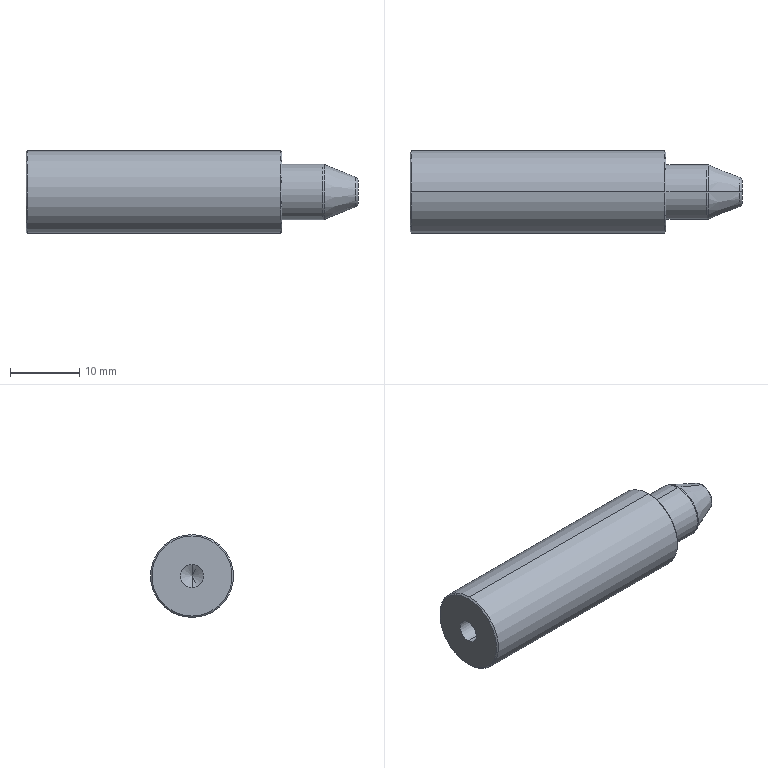Part | STEP file | 1 solid | 21 faces | box 48 x 12 x 12 mm | volume 4513 mm3 | cone 8 | cylinder 6 | torus 4 | plane 3 | commonest cylinder face diameters 3.3 x2 8 x2 12 x2
STEP:
#1=CARTESIAN_POINT('',(0.,0.,0.));
#2=DIRECTION('',(0.,0.,1.));
#3=DIRECTION('',(1.,0.,0.));
#4=AXIS2_PLACEMENT_3D('',#1,#2,#3);
#5=CARTESIAN_POINT('',(42.904,0.,4.));
#6=VERTEX_POINT('',#5);
#7=CARTESIAN_POINT('',(42.904,0.,-4.));
#8=VERTEX_POINT('',#7);
#9=CARTESIAN_POINT('',(42.904,0.,0.));
#10=DIRECTION('',(-1.,0.,0.));
#11=DIRECTION('',(0.,0.,-1.));
#12=AXIS2_PLACEMENT_3D('',#9,#10,#11);
#13=CIRCLE('',#12,4.);
#14=CARTESIAN_POINT('',(42.904,0.,0.));
#15=DIRECTION('',(1.,0.,0.));
#16=DIRECTION('',(0.,0.,-1.));
#17=AXIS2_PLACEMENT_3D('',#14,#15,#16);
#18=TOROIDAL_SURFACE('',#17,3.5,0.5);
#19=CARTESIAN_POINT('',(6.283,0.));
#20=DIRECTION('',(-1.,0.));
#21=VECTOR('',#20,1.);
#22=LINE('',#19,#21);
#23=(GEOMETRIC_REPRESENTATION_CONTEXT(2)PARAMETRIC_REPRESENTATION_CONTEXT()REPRESENTATION_CONTEXT('',''));
#24=DEFINITIONAL_REPRESENTATION('',(#22),#23);
#25=PCURVE('',#18,#24);
#26=CARTESIAN_POINT('',(0.,0.,0.));
#27=DIRECTION('',(-1.,0.,0.));
#28=DIRECTION('',(0.,0.,1.));
#29=AXIS2_PLACEMENT_3D('',#26,#27,#28);
#30=CYLINDRICAL_SURFACE('',#29,4.);
#31=CARTESIAN_POINT('',(-3.142,-42.904));
#32=DIRECTION('',(1.,0.));
#33=VECTOR('',#32,1.);
#34=LINE('',#31,#33);
#35=(GEOMETRIC_REPRESENTATION_CONTEXT(2)PARAMETRIC_REPRESENTATION_CONTEXT()REPRESENTATION_CONTEXT('',''));
#36=DEFINITIONAL_REPRESENTATION('',(#34),#35);
#37=PCURVE('',#30,#36);
#38=SURFACE_CURVE('',#13,(#25,#37),.PCURVE_S1.);
#39=EDGE_CURVE('',#6,#8,#38,.T.);
#40=ORIENTED_EDGE('',*,*,#39,.F.);
#41=CARTESIAN_POINT('',(43.089,0.,3.964));
#42=VERTEX_POINT('',#41);
#43=CARTESIAN_POINT('',(42.904,0.,3.5));
#44=DIRECTION('',(0.,1.,0.));
#45=DIRECTION('',(0.,0.,1.));
#46=AXIS2_PLACEMENT_3D('',#43,#44,#45);
#47=CIRCLE('',#46,0.5);
#48=CARTESIAN_POINT('',(3.142,0.));
#49=DIRECTION('',(0.,1.));
#50=VECTOR('',#49,1.);
#51=LINE('',#48,#50);
#52=(GEOMETRIC_REPRESENTATION_CONTEXT(2)PARAMETRIC_REPRESENTATION_CONTEXT()REPRESENTATION_CONTEXT('',''));
#53=DEFINITIONAL_REPRESENTATION('',(#51),#52);
#54=PCURVE('',#18,#53);
#55=CARTESIAN_POINT('',(42.904,0.,0.));
#56=DIRECTION('',(1.,0.,0.));
#57=DIRECTION('',(0.,0.,-1.));
#58=AXIS2_PLACEMENT_3D('',#55,#56,#57);
#59=TOROIDAL_SURFACE('',#58,3.5,0.5);
#60=CARTESIAN_POINT('',(3.142,0.));
#61=DIRECTION('',(0.,1.));
#62=VECTOR('',#61,1.);
#63=LINE('',#60,#62);
#64=(GEOMETRIC_REPRESENTATION_CONTEXT(2)PARAMETRIC_REPRESENTATION_CONTEXT()REPRESENTATION_CONTEXT('',''));
#65=DEFINITIONAL_REPRESENTATION('',(#63),#64);
#66=PCURVE('',#59,#65);
#67=SURFACE_CURVE('',#47,(#54,#66),.PCURVE_S1.);
#68=EDGE_CURVE('',#6,#42,#67,.T.);
#69=ORIENTED_EDGE('',*,*,#68,.T.);
#70=CARTESIAN_POINT('',(43.089,0.,-3.964));
#71=VERTEX_POINT('',#70);
#72=CARTESIAN_POINT('',(43.089,0.,0.));
#73=DIRECTION('',(1.,0.,0.));
#74=DIRECTION('',(0.,0.,1.));
#75=AXIS2_PLACEMENT_3D('',#72,#73,#74);
#76=CIRCLE('',#75,3.964);
#77=CARTESIAN_POINT('',(-3.142,0.3805));
#78=DIRECTION('',(1.,0.));
#79=VECTOR('',#78,1.);
#80=LINE('',#77,#79);
#81=(GEOMETRIC_REPRESENTATION_CONTEXT(2)PARAMETRIC_REPRESENTATION_CONTEXT()REPRESENTATION_CONTEXT('',''));
#82=DEFINITIONAL_REPRESENTATION('',(#80),#81);
#83=PCURVE('',#18,#82);
#84=CARTESIAN_POINT('',(43.,0.,0.));
#85=DIRECTION('',(-1.,0.,0.));
#86=DIRECTION('',(0.,0.,1.));
#87=AXIS2_PLACEMENT_3D('',#84,#85,#86);
#88=CONICAL_SURFACE('',#87,4.,0.3805);
#89=CARTESIAN_POINT('',(6.283,-0.0894));
#90=DIRECTION('',(-1.,0.));
#91=VECTOR('',#90,1.);
#92=LINE('',#89,#91);
#93=(GEOMETRIC_REPRESENTATION_CONTEXT(2)PARAMETRIC_REPRESENTATION_CONTEXT()REPRESENTATION_CONTEXT('',''));
#94=DEFINITIONAL_REPRESENTATION('',(#92),#93);
#95=PCURVE('',#88,#94);
#96=SURFACE_CURVE('',#76,(#83,#95),.PCURVE_S1.);
#97=EDGE_CURVE('',#71,#42,#96,.T.);
#98=ORIENTED_EDGE('',*,*,#97,.F.);
#99=CARTESIAN_POINT('',(42.904,0.,-3.5));
#100=DIRECTION('',(0.,-1.,0.));
#101=DIRECTION('',(0.,0.,-1.));
#102=AXIS2_PLACEMENT_3D('',#99,#100,#101);
#103=CIRCLE('',#102,0.5);
#104=CARTESIAN_POINT('',(0.,0.));
#105=DIRECTION('',(0.,1.));
#106=VECTOR('',#105,1.);
#107=LINE('',#104,#106);
#108=(GEOMETRIC_REPRESENTATION_CONTEXT(2)PARAMETRIC_REPRESENTATION_CONTEXT()REPRESENTATION_CONTEXT('',''));
#109=DEFINITIONAL_REPRESENTATION('',(#107),#108);
#110=PCURVE('',#18,#109);
#111=CARTESIAN_POINT('',(6.283,0.));
#112=DIRECTION('',(0.,1.));
#113=VECTOR('',#112,1.);
#114=LINE('',#111,#113);
#115=(GEOMETRIC_REPRESENTATION_CONTEXT(2)PARAMETRIC_REPRESENTATION_CONTEXT()REPRESENTATION_CONTEXT('',''));
#116=DEFINITIONAL_REPRESENTATION('',(#114),#115);
#117=PCURVE('',#59,#116);
#118=SURFACE_CURVE('',#103,(#110,#117),.PCURVE_S1.);
#119=EDGE_CURVE('',#8,#71,#118,.T.);
#120=ORIENTED_EDGE('',*,*,#119,.F.);
#121=EDGE_LOOP('',(#40,#69,#98,#120));
#122=FACE_BOUND('',#121,.T.);
#123=ADVANCED_FACE('',(#122),#18,.T.);
#124=CARTESIAN_POINT('',(48.,0.,-1.661));
#125=VERTEX_POINT('',#124);
#126=CARTESIAN_POINT('',(48.,0.,1.661));
#127=VERTEX_POINT('',#126);
#128=CARTESIAN_POINT('',(48.,0.,0.));
#129=DIRECTION('',(1.,0.,0.));
#130=DIRECTION('',(0.,0.,1.));
#131=AXIS2_PLACEMENT_3D('',#128,#129,#130);
#132=CIRCLE('',#131,1.661);
#133=CARTESIAN_POINT('',(47.5,0.,0.));
#134=DIRECTION('',(-1.,0.,0.));
#135=DIRECTION('',(0.,0.,1.));
#136=AXIS2_PLACEMENT_3D('',#133,#134,#135);
#137=TOROIDAL_SURFACE('',#136,1.661,0.5);
#138=CARTESIAN_POINT('',(6.283,4.712));
#139=DIRECTION('',(-1.,0.));
#140=VECTOR('',#139,1.);
#141=LINE('',#138,#140);
#142=(GEOMETRIC_REPRESENTATION_CONTEXT(2)PARAMETRIC_REPRESENTATION_CONTEXT()REPRESENTATION_CONTEXT('',''));
#143=DEFINITIONAL_REPRESENTATION('',(#141),#142);
#144=PCURVE('',#137,#143);
#145=CARTESIAN_POINT('',(48.,0.,0.));
#146=DIRECTION('',(-1.,0.,0.));
#147=DIRECTION('',(0.,0.,1.));
#148=AXIS2_PLACEMENT_3D('',#145,#146,#147);
#149=PLANE('',#148);
#150=CARTESIAN_POINT('',(1.661,0.));
#151=CARTESIAN_POINT('',(1.661,-2.878));
#152=CARTESIAN_POINT('',(-0.8307,-1.439));
#153=CARTESIAN_POINT('',(-3.323,0.));
#154=CARTESIAN_POINT('',(-0.8307,1.439));
#155=CARTESIAN_POINT('',(1.661,2.878));
#156=CARTESIAN_POINT('',(1.661,0.));
#157=(BOUNDED_CURVE()B_SPLINE_CURVE(2,(#150,#151,#152,#153,#154,#155,#156),.UNSPECIFIED.,.T.,.F.)B_SPLINE_CURVE_WITH_KNOTS((1,2,2,2,2,1),(-2.094,0.,2.094,4.189,6.283,8.378),.UNSPECIFIED.)CURVE()GEOMETRIC_REPRESENTATION_ITEM()RATIONAL_B_SPLINE_CURVE((1.,0.5,1.,0.5,1.,0.5,1.))REPRESENTATION_ITEM(''));
#158=(GEOMETRIC_REPRESENTATION_CONTEXT(2)PARAMETRIC_REPRESENTATION_CONTEXT()REPRESENTATION_CONTEXT('',''));
#159=DEFINITIONAL_REPRESENTATION('',(#157),#158);
#160=PCURVE('',#149,#159);
#161=SURFACE_CURVE('',#132,(#144,#160),.PCURVE_S1.);
#162=EDGE_CURVE('',#125,#127,#161,.T.);
#163=ORIENTED_EDGE('',*,*,#162,.F.);
#164=CARTESIAN_POINT('',(47.686,0.,-2.126));
#165=VERTEX_POINT('',#164);
#166=CARTESIAN_POINT('',(47.5,0.,-1.661));
#167=DIRECTION('',(0.,1.,0.));
#168=DIRECTION('',(0.,0.,1.));
#169=AXIS2_PLACEMENT_3D('',#166,#167,#168);
#170=CIRCLE('',#169,0.5);
#171=CARTESIAN_POINT('',(3.142,3.142));
#172=DIRECTION('',(0.,1.));
#173=VECTOR('',#172,1.);
#174=LINE('',#171,#173);
#175=(GEOMETRIC_REPRESENTATION_CONTEXT(2)PARAMETRIC_REPRESENTATION_CONTEXT()REPRESENTATION_CONTEXT('',''));
#176=DEFINITIONAL_REPRESENTATION('',(#174),#175);
#177=PCURVE('',#137,#176);
#178=CARTESIAN_POINT('',(47.5,0.,0.));
#179=DIRECTION('',(-1.,0.,0.));
#180=DIRECTION('',(0.,0.,1.));
#181=AXIS2_PLACEMENT_3D('',#178,#179,#180);
#182=TOROIDAL_SURFACE('',#181,1.661,0.5);
#183=CARTESIAN_POINT('',(3.142,3.142));
#184=DIRECTION('',(0.,1.));
#185=VECTOR('',#184,1.);
#186=LINE('',#183,#185);
#187=(GEOMETRIC_REPRESENTATION_CONTEXT(2)PARAMETRIC_REPRESENTATION_CONTEXT()REPRESENTATION_CONTEXT('',''));
#188=DEFINITIONAL_REPRESENTATION('',(#186),#187);
#189=PCURVE('',#182,#188);
#190=SURFACE_CURVE('',#170,(#177,#189),.PCURVE_S1.);
#191=EDGE_CURVE('',#125,#165,#190,.T.);
#192=ORIENTED_EDGE('',*,*,#191,.T.);
#193=CARTESIAN_POINT('',(47.686,0.,2.126));
#194=VERTEX_POINT('',#193);
#195=CARTESIAN_POINT('',(47.686,0.,0.));
#196=DIRECTION('',(-1.,0.,0.));
#197=DIRECTION('',(0.,0.,1.));
#198=AXIS2_PLACEMENT_3D('',#195,#196,#197);
#199=CIRCLE('',#198,2.126);
#200=CARTESIAN_POINT('',(0.,5.903));
#201=DIRECTION('',(1.,0.));
#202=VECTOR('',#201,1.);
#203=LINE('',#200,#202);
#204=(GEOMETRIC_REPRESENTATION_CONTEXT(2)PARAMETRIC_REPRESENTATION_CONTEXT()REPRESENTATION_CONTEXT('',''));
#205=DEFINITIONAL_REPRESENTATION('',(#203),#204);
#206=PCURVE('',#137,#205);
#207=CARTESIAN_POINT('',(0.,-4.686));
#208=DIRECTION('',(1.,0.));
#209=VECTOR('',#208,1.);
#210=LINE('',#207,#209);
#211=(GEOMETRIC_REPRESENTATION_CONTEXT(2)PARAMETRIC_REPRESENTATION_CONTEXT()REPRESENTATION_CONTEXT('',''));
#212=DEFINITIONAL_REPRESENTATION('',(#210),#211);
#213=PCURVE('',#88,#212);
#214=SURFACE_CURVE('',#199,(#206,#213),.PCURVE_S1.);
#215=EDGE_CURVE('',#194,#165,#214,.T.);
#216=ORIENTED_EDGE('',*,*,#215,.F.);
#217=CARTESIAN_POINT('',(47.5,0.,1.661));
#218=DIRECTION('',(0.,-1.,0.));
#219=DIRECTION('',(0.,0.,-1.));
#220=AXIS2_PLACEMENT_3D('',#217,#218,#219);
#221=CIRCLE('',#220,0.5);
#222=CARTESIAN_POINT('',(0.,3.142));
#223=DIRECTION('',(0.,1.));
#224=VECTOR('',#223,1.);
#225=LINE('',#222,#224);
#226=(GEOMETRIC_REPRESENTATION_CONTEXT(2)PARAMETRIC_REPRESENTATION_CONTEXT()REPRESENTATION_CONTEXT('',''));
#227=DEFINITIONAL_REPRESENTATION('',(#225),#226);
#228=PCURVE('',#137,#227);
#229=CARTESIAN_POINT('',(6.283,3.142));
#230=DIRECTION('',(0.,1.));
#231=VECTOR('',#230,1.);
#232=LINE('',#229,#231);
#233=(GEOMETRIC_REPRESENTATION_CONTEXT(2)PARAMETRIC_REPRESENTATION_CONTEXT()REPRESENTATION_CONTEXT('',''));
#234=DEFINITIONAL_REPRESENTATION('',(#232),#233);
#235=PCURVE('',#182,#234);
#236=SURFACE_CURVE('',#221,(#228,#235),.PCURVE_S1.);
#237=EDGE_CURVE('',#127,#194,#236,.T.);
#238=ORIENTED_EDGE('',*,*,#237,.F.);
#239=EDGE_LOOP('',(#163,#192,#216,#238));
#240=FACE_BOUND('',#239,.T.);
#241=ADVANCED_FACE('',(#240),#137,.T.);
#242=CARTESIAN_POINT('',(37.,0.,-5.8));
#243=VERTEX_POINT('',#242);
#244=CARTESIAN_POINT('',(37.,0.,5.8));
#245=VERTEX_POINT('',#244);
#246=CARTESIAN_POINT('',(37.,0.,0.));
#247=DIRECTION('',(1.,0.,0.));
#248=DIRECTION('',(0.,0.,1.));
#249=AXIS2_PLACEMENT_3D('',#246,#247,#248);
#250=CIRCLE('',#249,5.8);
#251=CARTESIAN_POINT('',(36.8,0.,0.));
#252=DIRECTION('',(-1.,0.,0.));
#253=DIRECTION('',(0.,0.,1.));
#254=AXIS2_PLACEMENT_3D('',#251,#252,#253);
#255=CONICAL_SURFACE('',#254,6.,0.7854);
#256=CARTESIAN_POINT('',(6.283,-0.2));
#257=DIRECTION('',(-1.,0.));
#258=VECTOR('',#257,1.);
#259=LINE('',#256,#258);
#260=(GEOMETRIC_REPRESENTATION_CONTEXT(2)PARAMETRIC_REPRESENTATION_CONTEXT()REPRESENTATION_CONTEXT('',''));
#261=DEFINITIONAL_REPRESENTATION('',(#259),#260);
#262=PCURVE('',#255,#261);
#263=CARTESIAN_POINT('',(37.,4.,0.));
#264=DIRECTION('',(-1.,0.,0.));
#265=DIRECTION('',(0.,0.,1.));
#266=AXIS2_PLACEMENT_3D('',#263,#264,#265);
#267=PLANE('',#266);
#268=CARTESIAN_POINT('',(5.8,-4.));
#269=CARTESIAN_POINT('',(5.8,-14.046));
#270=CARTESIAN_POINT('',(-2.9,-9.023));
#271=CARTESIAN_POINT('',(-11.6,-4.));
#272=CARTESIAN_POINT('',(-2.9,1.023));
#273=CARTESIAN_POINT('',(5.8,6.046));
#274=CARTESIAN_POINT('',(5.8,-4.));
#275=(BOUNDED_CURVE()B_SPLINE_CURVE(2,(#268,#269,#270,#271,#272,#273,#274),.UNSPECIFIED.,.T.,.F.)B_SPLINE_CURVE_WITH_KNOTS((1,2,2,2,2,1),(-2.094,0.,2.094,4.189,6.283,8.378),.UNSPECIFIED.)CURVE()GEOMETRIC_REPRESENTATION_ITEM()RATIONAL_B_SPLINE_CURVE((1.,0.5,1.,0.5,1.,0.5,1.))REPRESENTATION_ITEM(''));
#276=(GEOMETRIC_REPRESENTATION_CONTEXT(2)PARAMETRIC_REPRESENTATION_CONTEXT()REPRESENTATION_CONTEXT('',''));
#277=DEFINITIONAL_REPRESENTATION('',(#275),#276);
#278=PCURVE('',#267,#277);
#279=SURFACE_CURVE('',#250,(#262,#278),.PCURVE_S1.);
#280=EDGE_CURVE('',#243,#245,#279,.T.);
#281=ORIENTED_EDGE('',*,*,#280,.F.);
#282=CARTESIAN_POINT('',(36.8,0.,-6.));
#283=VERTEX_POINT('',#282);
#284=CARTESIAN_POINT('',(36.8,0.,-6.));
#285=DIRECTION('',(-0.7071,0.,-0.7071));
#286=VECTOR('',#285,1.);
#287=LINE('',#284,#286);
#288=CARTESIAN_POINT('',(3.142,0.));
#289=DIRECTION('',(0.,1.));
#290=VECTOR('',#289,1.);
#291=LINE('',#288,#290);
#292=(GEOMETRIC_REPRESENTATION_CONTEXT(2)PARAMETRIC_REPRESENTATION_CONTEXT()REPRESENTATION_CONTEXT('',''));
#293=DEFINITIONAL_REPRESENTATION('',(#291),#292);
#294=PCURVE('',#255,#293);
#295=CARTESIAN_POINT('',(36.8,0.,0.));
#296=DIRECTION('',(-1.,0.,0.));
#297=DIRECTION('',(0.,0.,1.));
#298=AXIS2_PLACEMENT_3D('',#295,#296,#297);
#299=CONICAL_SURFACE('',#298,6.,0.7854);
#300=CARTESIAN_POINT('',(3.142,0.));
#301=DIRECTION('',(0.,1.));
#302=VECTOR('',#301,1.);
#303=LINE('',#300,#302);
#304=(GEOMETRIC_REPRESENTATION_CONTEXT(2)PARAMETRIC_REPRESENTATION_CONTEXT()REPRESENTATION_CONTEXT('',''));
#305=DEFINITIONAL_REPRESENTATION('',(#303),#304);
#306=PCURVE('',#299,#305);
#307=SURFACE_CURVE('',#287,(#294,#306),.PCURVE_S1.);
#308=EDGE_CURVE('',#243,#283,#307,.T.);
#309=ORIENTED_EDGE('',*,*,#308,.T.);
#310=CARTESIAN_POINT('',(36.8,0.,6.));
#311=VERTEX_POINT('',#310);
#312=CARTESIAN_POINT('',(36.8,0.,0.));
#313=DIRECTION('',(-1.,0.,0.));
#314=DIRECTION('',(0.,0.,1.));
#315=AXIS2_PLACEMENT_3D('',#312,#313,#314);
#316=CIRCLE('',#315,6.);
#317=CARTESIAN_POINT('',(0.,0.));
#318=DIRECTION('',(1.,0.));
#319=VECTOR('',#318,1.);
#320=LINE('',#317,#319);
#321=(GEOMETRIC_REPRESENTATION_CONTEXT(2)PARAMETRIC_REPRESENTATION_CONTEXT()REPRESENTATION_CONTEXT('',''));
#322=DEFINITIONAL_REPRESENTATION('',(#320),#321);
#323=PCURVE('',#255,#322);
#324=CARTESIAN_POINT('',(0.,0.,0.));
#325=DIRECTION('',(-1.,0.,0.));
#326=DIRECTION('',(0.,0.,1.));
#327=AXIS2_PLACEMENT_3D('',#324,#325,#326);
#328=CYLINDRICAL_SURFACE('',#327,6.);
#329=CARTESIAN_POINT('',(0.,-36.8));
#330=DIRECTION('',(1.,0.));
#331=VECTOR('',#330,1.);
#332=LINE('',#329,#331);
#333=(GEOMETRIC_REPRESENTATION_CONTEXT(2)PARAMETRIC_REPRESENTATION_CONTEXT()REPRESENTATION_CONTEXT('',''));
#334=DEFINITIONAL_REPRESENTATION('',(#332),#333);
#335=PCURVE('',#328,#334);
#336=SURFACE_CURVE('',#316,(#323,#335),.PCURVE_S1.);
#337=EDGE_CURVE('',#311,#283,#336,.T.);
#338=ORIENTED_EDGE('',*,*,#337,.F.);
#339=CARTESIAN_POINT('',(36.8,0.,6.));
#340=DIRECTION('',(-0.7071,0.,0.7071));
#341=VECTOR('',#340,1.);
#342=LINE('',#339,#341);
#343=CARTESIAN_POINT('',(0.,0.));
#344=DIRECTION('',(0.,1.));
#345=VECTOR('',#344,1.);
#346=LINE('',#343,#345);
#347=(GEOMETRIC_REPRESENTATION_CONTEXT(2)PARAMETRIC_REPRESENTATION_CONTEXT()REPRESENTATION_CONTEXT('',''));
#348=DEFINITIONAL_REPRESENTATION('',(#346),#347);
#349=PCURVE('',#255,#348);
#350=CARTESIAN_POINT('',(6.283,0.));
#351=DIRECTION('',(0.,1.));
#352=VECTOR('',#351,1.);
#353=LINE('',#350,#352);
#354=(GEOMETRIC_REPRESENTATION_CONTEXT(2)PARAMETRIC_REPRESENTATION_CONTEXT()REPRESENTATION_CONTEXT('',''));
#355=DEFINITIONAL_REPRESENTATION('',(#353),#354);
#356=PCURVE('',#299,#355);
#357=SURFACE_CURVE('',#342,(#349,#356),.PCURVE_S1.);
#358=EDGE_CURVE('',#245,#311,#357,.T.);
#359=ORIENTED_EDGE('',*,*,#358,.F.);
#360=EDGE_LOOP('',(#281,#309,#338,#359));
#361=FACE_BOUND('',#360,.T.);
#362=ADVANCED_FACE('',(#361),#255,.T.);
#363=CARTESIAN_POINT('',(0.,0.,5.8));
#364=VERTEX_POINT('',#363);
#365=CARTESIAN_POINT('',(0.,0.,-5.8));
#366=VERTEX_POINT('',#365);
#367=CARTESIAN_POINT('',(0.,0.,0.));
#368=DIRECTION('',(-1.,0.,0.));
#369=DIRECTION('',(0.,0.,-1.));
#370=AXIS2_PLACEMENT_3D('',#367,#368,#369);
#371=CIRCLE('',#370,5.8);
#372=CARTESIAN_POINT('',(0.,0.,0.));
#373=DIRECTION('',(1.,0.,0.));
#374=DIRECTION('',(0.,0.,-1.));
#375=AXIS2_PLACEMENT_3D('',#372,#373,#374);
#376=CONICAL_SURFACE('',#375,5.8,0.7854);
#377=CARTESIAN_POINT('',(6.283,0.));
#378=DIRECTION('',(-1.,0.));
#379=VECTOR('',#378,1.);
#380=LINE('',#377,#379);
#381=(GEOMETRIC_REPRESENTATION_CONTEXT(2)PARAMETRIC_REPRESENTATION_CONTEXT()REPRESENTATION_CONTEXT('',''));
#382=DEFINITIONAL_REPRESENTATION('',(#380),#381);
#383=PCURVE('',#376,#382);
#384=CARTESIAN_POINT('',(0.,6.,0.));
#385=DIRECTION('',(1.,0.,0.));
#386=DIRECTION('',(0.,0.,-1.));
#387=AXIS2_PLACEMENT_3D('',#384,#385,#386);
#388=PLANE('',#387);
#389=CARTESIAN_POINT('',(5.8,-6.));
#390=CARTESIAN_POINT('',(5.8,-16.046));
#391=CARTESIAN_POINT('',(-2.9,-11.023));
#392=CARTESIAN_POINT('',(-11.6,-6.));
#393=CARTESIAN_POINT('',(-2.9,-0.9771));
#394=CARTESIAN_POINT('',(5.8,4.046));
#395=CARTESIAN_POINT('',(5.8,-6.));
#396=(BOUNDED_CURVE()B_SPLINE_CURVE(2,(#389,#390,#391,#392,#393,#394,#395),.UNSPECIFIED.,.T.,.F.)B_SPLINE_CURVE_WITH_KNOTS((1,2,2,2,2,1),(-2.094,0.,2.094,4.189,6.283,8.378),.UNSPECIFIED.)CURVE()GEOMETRIC_REPRESENTATION_ITEM()RATIONAL_B_SPLINE_CURVE((1.,0.5,1.,0.5,1.,0.5,1.))REPRESENTATION_ITEM(''));
#397=(GEOMETRIC_REPRESENTATION_CONTEXT(2)PARAMETRIC_REPRESENTATION_CONTEXT()REPRESENTATION_CONTEXT('',''));
#398=DEFINITIONAL_REPRESENTATION('',(#396),#397);
#399=PCURVE('',#388,#398);
#400=SURFACE_CURVE('',#371,(#383,#399),.PCURVE_S1.);
#401=EDGE_CURVE('',#364,#366,#400,.T.);
#402=ORIENTED_EDGE('',*,*,#401,.F.);
#403=CARTESIAN_POINT('',(0.2,0.,6.));
#404=VERTEX_POINT('',#403);
#405=CARTESIAN_POINT('',(0.,0.,5.8));
#406=DIRECTION('',(0.7071,0.,0.7071));
#407=VECTOR('',#406,1.);
#408=LINE('',#405,#407);
#409=CARTESIAN_POINT('',(3.142,0.));
#410=DIRECTION('',(0.,1.));
#411=VECTOR('',#410,1.);
#412=LINE('',#409,#411);
#413=(GEOMETRIC_REPRESENTATION_CONTEXT(2)PARAMETRIC_REPRESENTATION_CONTEXT()REPRESENTATION_CONTEXT('',''));
#414=DEFINITIONAL_REPRESENTATION('',(#412),#413);
#415=PCURVE('',#376,#414);
#416=CARTESIAN_POINT('',(0.,0.,0.));
#417=DIRECTION('',(1.,0.,0.));
#418=DIRECTION('',(0.,0.,-1.));
#419=AXIS2_PLACEMENT_3D('',#416,#417,#418);
#420=CONICAL_SURFACE('',#419,5.8,0.7854);
#421=CARTESIAN_POINT('',(3.142,0.));
#422=DIRECTION('',(0.,1.));
#423=VECTOR('',#422,1.);
#424=LINE('',#421,#423);
#425=(GEOMETRIC_REPRESENTATION_CONTEXT(2)PARAMETRIC_REPRESENTATION_CONTEXT()REPRESENTATION_CONTEXT('',''));
#426=DEFINITIONAL_REPRESENTATION('',(#424),#425);
#427=PCURVE('',#420,#426);
#428=SURFACE_CURVE('',#408,(#415,#427),.PCURVE_S1.);
#429=EDGE_CURVE('',#364,#404,#428,.T.);
#430=ORIENTED_EDGE('',*,*,#429,.T.);
#431=CARTESIAN_POINT('',(0.2,0.,-6.));
#432=VERTEX_POINT('',#431);
#433=CARTESIAN_POINT('',(0.2,0.,0.));
#434=DIRECTION('',(1.,0.,0.));
#435=DIRECTION('',(0.,0.,-1.));
#436=AXIS2_PLACEMENT_3D('',#433,#434,#435);
#437=CIRCLE('',#436,6.);
#438=CARTESIAN_POINT('',(0.,0.2));
#439=DIRECTION('',(1.,0.));
#440=VECTOR('',#439,1.);
#441=LINE('',#438,#440);
#442=(GEOMETRIC_REPRESENTATION_CONTEXT(2)PARAMETRIC_REPRESENTATION_CONTEXT()REPRESENTATION_CONTEXT('',''));
#443=DEFINITIONAL_REPRESENTATION('',(#441),#442);
#444=PCURVE('',#376,#443);
#445=CARTESIAN_POINT('',(3.142,-0.2));
#446=DIRECTION('',(-1.,0.));
#447=VECTOR('',#446,1.);
#448=LINE('',#445,#447);
#449=(GEOMETRIC_REPRESENTATION_CONTEXT(2)PARAMETRIC_REPRESENTATION_CONTEXT()REPRESENTATION_CONTEXT('',''));
#450=DEFINITIONAL_REPRESENTATION('',(#448),#449);
#451=PCURVE('',#328,#450);
#452=SURFACE_CURVE('',#437,(#444,#451),.PCURVE_S1.);
#453=EDGE_CURVE('',#432,#404,#452,.T.);
#454=ORIENTED_EDGE('',*,*,#453,.F.);
#455=CARTESIAN_POINT('',(0.,0.,-5.8));
#456=DIRECTION('',(0.7071,0.,-0.7071));
#457=VECTOR('',#456,1.);
#458=LINE('',#455,#457);
#459=CARTESIAN_POINT('',(0.,0.));
#460=DIRECTION('',(0.,1.));
#461=VECTOR('',#460,1.);
#462=LINE('',#459,#461);
#463=(GEOMETRIC_REPRESENTATION_CONTEXT(2)PARAMETRIC_REPRESENTATION_CONTEXT()REPRESENTATION_CONTEXT('',''));
#464=DEFINITIONAL_REPRESENTATION('',(#462),#463);
#465=PCURVE('',#376,#464);
#466=CARTESIAN_POINT('',(6.283,0.));
#467=DIRECTION('',(0.,1.));
#468=VECTOR('',#467,1.);
#469=LINE('',#466,#468);
#470=(GEOMETRIC_REPRESENTATION_CONTEXT(2)PARAMETRIC_REPRESENTATION_CONTEXT()REPRESENTATION_CONTEXT('',''));
#471=DEFINITIONAL_REPRESENTATION('',(#469),#470);
#472=PCURVE('',#420,#471);
#473=SURFACE_CURVE('',#458,(#465,#472),.PCURVE_S1.);
#474=EDGE_CURVE('',#366,#432,#473,.T.);
#475=ORIENTED_EDGE('',*,*,#474,.F.);
#476=EDGE_LOOP('',(#402,#430,#454,#475));
#477=FACE_BOUND('',#476,.T.);
#478=ADVANCED_FACE('',(#477),#376,.T.);
#479=ORIENTED_EDGE('',*,*,#215,.T.);
#480=CARTESIAN_POINT('',(43.,0.,-4.));
#481=DIRECTION('',(-0.9285,0.,-0.3714));
#482=VECTOR('',#481,1.);
#483=LINE('',#480,#482);
#484=CARTESIAN_POINT('',(3.142,0.));
#485=DIRECTION('',(0.,1.));
#486=VECTOR('',#485,1.);
#487=LINE('',#484,#486);
#488=(GEOMETRIC_REPRESENTATION_CONTEXT(2)PARAMETRIC_REPRESENTATION_CONTEXT()REPRESENTATION_CONTEXT('',''));
#489=DEFINITIONAL_REPRESENTATION('',(#487),#488);
#490=PCURVE('',#88,#489);
#491=CARTESIAN_POINT('',(43.,0.,0.));
#492=DIRECTION('',(-1.,0.,0.));
#493=DIRECTION('',(0.,0.,1.));
#494=AXIS2_PLACEMENT_3D('',#491,#492,#493);
#495=CONICAL_SURFACE('',#494,4.,0.3805);
#496=CARTESIAN_POINT('',(3.142,0.));
#497=DIRECTION('',(0.,1.));
#498=VECTOR('',#497,1.);
#499=LINE('',#496,#498);
#500=(GEOMETRIC_REPRESENTATION_CONTEXT(2)PARAMETRIC_REPRESENTATION_CONTEXT()REPRESENTATION_CONTEXT('',''));
#501=DEFINITIONAL_REPRESENTATION('',(#499),#500);
#502=PCURVE('',#495,#501);
#503=SURFACE_CURVE('',#483,(#490,#502),.PCURVE_S1.);
#504=EDGE_CURVE('',#165,#71,#503,.T.);
#505=ORIENTED_EDGE('',*,*,#504,.T.);
#506=ORIENTED_EDGE('',*,*,#97,.T.);
#507=CARTESIAN_POINT('',(43.,0.,4.));
#508=DIRECTION('',(-0.9285,0.,0.3714));
#509=VECTOR('',#508,1.);
#510=LINE('',#507,#509);
#511=CARTESIAN_POINT('',(0.,0.));
#512=DIRECTION('',(0.,1.));
#513=VECTOR('',#512,1.);
#514=LINE('',#511,#513);
#515=(GEOMETRIC_REPRESENTATION_CONTEXT(2)PARAMETRIC_REPRESENTATION_CONTEXT()REPRESENTATION_CONTEXT('',''));
#516=DEFINITIONAL_REPRESENTATION('',(#514),#515);
#517=PCURVE('',#88,#516);
#518=CARTESIAN_POINT('',(6.283,0.));
#519=DIRECTION('',(0.,1.));
#520=VECTOR('',#519,1.);
#521=LINE('',#518,#520);
#522=(GEOMETRIC_REPRESENTATION_CONTEXT(2)PARAMETRIC_REPRESENTATION_CONTEXT()REPRESENTATION_CONTEXT('',''));
#523=DEFINITIONAL_REPRESENTATION('',(#521),#522);
#524=PCURVE('',#495,#523);
#525=SURFACE_CURVE('',#510,(#517,#524),.PCURVE_S1.);
#526=EDGE_CURVE('',#194,#42,#525,.T.);
#527=ORIENTED_EDGE('',*,*,#526,.F.);
#528=EDGE_LOOP('',(#479,#505,#506,#527));
#529=FACE_BOUND('',#528,.T.);
#530=ADVANCED_FACE('',(#529),#88,.T.);
#531=CARTESIAN_POINT('',(13.5,0.,1.65));
#532=VERTEX_POINT('',#531);
#533=CARTESIAN_POINT('',(0.,0.,1.65));
#534=VERTEX_POINT('',#533);
#535=CARTESIAN_POINT('',(0.,0.,1.65));
#536=DIRECTION('',(-1.,0.,0.));
#537=VECTOR('',#536,1.);
#538=LINE('',#535,#537);
#539=CARTESIAN_POINT('',(0.,0.,0.));
#540=DIRECTION('',(-1.,0.,0.));
#541=DIRECTION('',(0.,0.,1.));
#542=AXIS2_PLACEMENT_3D('',#539,#540,#541);
#543=CYLINDRICAL_SURFACE('',#542,1.65);
#544=CARTESIAN_POINT('',(6.283,0.));
#545=DIRECTION('',(0.,1.));
#546=VECTOR('',#545,1.);
#547=LINE('',#544,#546);
#548=(GEOMETRIC_REPRESENTATION_CONTEXT(2)PARAMETRIC_REPRESENTATION_CONTEXT()REPRESENTATION_CONTEXT('',''));
#549=DEFINITIONAL_REPRESENTATION('',(#547),#548);
#550=PCURVE('',#543,#549);
#551=CARTESIAN_POINT('',(0.,0.,0.));
#552=DIRECTION('',(-1.,0.,0.));
#553=DIRECTION('',(0.,0.,1.));
#554=AXIS2_PLACEMENT_3D('',#551,#552,#553);
#555=CYLINDRICAL_SURFACE('',#554,1.65);
#556=CARTESIAN_POINT('',(0.,0.));
#557=DIRECTION('',(0.,1.));
#558=VECTOR('',#557,1.);
#559=LINE('',#556,#558);
#560=(GEOMETRIC_REPRESENTATION_CONTEXT(2)PARAMETRIC_REPRESENTATION_CONTEXT()REPRESENTATION_CONTEXT('',''));
#561=DEFINITIONAL_REPRESENTATION('',(#559),#560);
#562=PCURVE('',#555,#561);
#563=SURFACE_CURVE('',#538,(#550,#562),.PCURVE_S1.);
#564=EDGE_CURVE('',#532,#534,#563,.T.);
#565=ORIENTED_EDGE('',*,*,#564,.T.);
#566=CARTESIAN_POINT('',(0.,0.,-1.65));
#567=VERTEX_POINT('',#566);
#568=CARTESIAN_POINT('',(0.,0.,0.));
#569=DIRECTION('',(-1.,0.,0.));
#570=DIRECTION('',(0.,0.,1.));
#571=AXIS2_PLACEMENT_3D('',#568,#569,#570);
#572=CIRCLE('',#571,1.65);
#573=CARTESIAN_POINT('',(0.,0.));
#574=DIRECTION('',(1.,0.));
#575=VECTOR('',#574,1.);
#576=LINE('',#573,#575);
#577=(GEOMETRIC_REPRESENTATION_CONTEXT(2)PARAMETRIC_REPRESENTATION_CONTEXT()REPRESENTATION_CONTEXT('',''));
#578=DEFINITIONAL_REPRESENTATION('',(#576),#577);
#579=PCURVE('',#543,#578);
#580=CARTESIAN_POINT('',(-1.65,-6.));
#581=CARTESIAN_POINT('',(-1.65,-3.142));
#582=CARTESIAN_POINT('',(0.825,-4.571));
#583=CARTESIAN_POINT('',(3.3,-6.));
#584=CARTESIAN_POINT('',(0.825,-7.429));
#585=CARTESIAN_POINT('',(-1.65,-8.858));
#586=CARTESIAN_POINT('',(-1.65,-6.));
#587=(BOUNDED_CURVE()B_SPLINE_CURVE(2,(#580,#581,#582,#583,#584,#585,#586),.UNSPECIFIED.,.T.,.F.)B_SPLINE_CURVE_WITH_KNOTS((1,2,2,2,2,1),(-2.094,0.,2.094,4.189,6.283,8.378),.UNSPECIFIED.)CURVE()GEOMETRIC_REPRESENTATION_ITEM()RATIONAL_B_SPLINE_CURVE((1.,0.5,1.,0.5,1.,0.5,1.))REPRESENTATION_ITEM(''));
#588=(GEOMETRIC_REPRESENTATION_CONTEXT(2)PARAMETRIC_REPRESENTATION_CONTEXT()REPRESENTATION_CONTEXT('',''));
#589=DEFINITIONAL_REPRESENTATION('',(#587),#588);
#590=PCURVE('',#388,#589);
#591=SURFACE_CURVE('',#572,(#579,#590),.PCURVE_S1.);
#592=EDGE_CURVE('',#567,#534,#591,.T.);
#593=ORIENTED_EDGE('',*,*,#592,.F.);
#594=CARTESIAN_POINT('',(13.5,0.,-1.65));
#595=VERTEX_POINT('',#594);
#596=CARTESIAN_POINT('',(0.,0.,-1.65));
#597=DIRECTION('',(-1.,0.,0.));
#598=VECTOR('',#597,1.);
#599=LINE('',#596,#598);
#600=CARTESIAN_POINT('',(3.142,0.));
#601=DIRECTION('',(0.,1.));
#602=VECTOR('',#601,1.);
#603=LINE('',#600,#602);
#604=(GEOMETRIC_REPRESENTATION_CONTEXT(2)PARAMETRIC_REPRESENTATION_CONTEXT()REPRESENTATION_CONTEXT('',''));
#605=DEFINITIONAL_REPRESENTATION('',(#603),#604);
#606=PCURVE('',#543,#605);
#607=CARTESIAN_POINT('',(3.142,0.));
#608=DIRECTION('',(0.,1.));
#609=VECTOR('',#608,1.);
#610=LINE('',#607,#609);
#611=(GEOMETRIC_REPRESENTATION_CONTEXT(2)PARAMETRIC_REPRESENTATION_CONTEXT()REPRESENTATION_CONTEXT('',''));
#612=DEFINITIONAL_REPRESENTATION('',(#610),#611);
#613=PCURVE('',#555,#612);
#614=SURFACE_CURVE('',#599,(#606,#613),.PCURVE_S1.);
#615=EDGE_CURVE('',#595,#567,#614,.T.);
#616=ORIENTED_EDGE('',*,*,#615,.F.);
#617=CARTESIAN_POINT('',(13.5,0.,0.));
#618=DIRECTION('',(-1.,0.,0.));
#619=DIRECTION('',(0.,0.,1.));
#620=AXIS2_PLACEMENT_3D('',#617,#618,#619);
#621=CIRCLE('',#620,1.65);
#622=CARTESIAN_POINT('',(0.,-13.5));
#623=DIRECTION('',(1.,0.));
#624=VECTOR('',#623,1.);
#625=LINE('',#622,#624);
#626=(GEOMETRIC_REPRESENTATION_CONTEXT(2)PARAMETRIC_REPRESENTATION_CONTEXT()REPRESENTATION_CONTEXT('',''));
#627=DEFINITIONAL_REPRESENTATION('',(#625),#626);
#628=PCURVE('',#543,#627);
#629=CARTESIAN_POINT('',(13.5,0.,0.));
#630=DIRECTION('',(-1.,0.,0.));
#631=DIRECTION('',(0.,0.,1.));
#632=AXIS2_PLACEMENT_3D('',#629,#630,#631);
#633=CONICAL_SURFACE('',#632,1.65,1.03);
#634=CARTESIAN_POINT('',(0.,0.));
#635=DIRECTION('',(1.,0.));
#636=VECTOR('',#635,1.);
#637=LINE('',#634,#636);
#638=(GEOMETRIC_REPRESENTATION_CONTEXT(2)PARAMETRIC_REPRESENTATION_CONTEXT()REPRESENTATION_CONTEXT('',''));
#639=DEFINITIONAL_REPRESENTATION('',(#637),#638);
#640=PCURVE('',#633,#639);
#641=SURFACE_CURVE('',#621,(#628,#640),.PCURVE_S1.);
#642=EDGE_CURVE('',#595,#532,#641,.T.);
#643=ORIENTED_EDGE('',*,*,#642,.T.);
#644=EDGE_LOOP('',(#565,#593,#616,#643));
#645=FACE_BOUND('',#644,.F.);
#646=ADVANCED_FACE('',(#645),#543,.F.);
#647=ORIENTED_EDGE('',*,*,#642,.F.);
#648=CARTESIAN_POINT('',(14.491,0.,0.));
#649=VERTEX_POINT('',#648);
#650=CARTESIAN_POINT('',(13.5,0.,-1.65));
#651=DIRECTION('',(-0.515,0.,-0.8572));
#652=VECTOR('',#651,1.);
#653=LINE('',#650,#652);
#654=CARTESIAN_POINT('',(3.142,0.));
#655=DIRECTION('',(0.,1.));
#656=VECTOR('',#655,1.);
#657=LINE('',#654,#656);
#658=(GEOMETRIC_REPRESENTATION_CONTEXT(2)PARAMETRIC_REPRESENTATION_CONTEXT()REPRESENTATION_CONTEXT('',''));
#659=DEFINITIONAL_REPRESENTATION('',(#657),#658);
#660=PCURVE('',#633,#659);
#661=CARTESIAN_POINT('',(13.5,0.,0.));
#662=DIRECTION('',(-1.,0.,0.));
#663=DIRECTION('',(0.,0.,1.));
#664=AXIS2_PLACEMENT_3D('',#661,#662,#663);
#665=CONICAL_SURFACE('',#664,1.65,1.03);
#666=CARTESIAN_POINT('',(3.142,0.));
#667=DIRECTION('',(0.,1.));
#668=VECTOR('',#667,1.);
#669=LINE('',#666,#668);
#670=(GEOMETRIC_REPRESENTATION_CONTEXT(2)PARAMETRIC_REPRESENTATION_CONTEXT()REPRESENTATION_CONTEXT('',''));
#671=DEFINITIONAL_REPRESENTATION('',(#669),#670);
#672=PCURVE('',#665,#671);
#673=SURFACE_CURVE('',#653,(#660,#672),.PCURVE_S1.);
#674=EDGE_CURVE('',#649,#595,#673,.T.);
#675=ORIENTED_EDGE('',*,*,#674,.F.);
#676=CARTESIAN_POINT('',(13.5,0.,1.65));
#677=DIRECTION('',(-0.515,0.,0.8572));
#678=VECTOR('',#677,1.);
#679=LINE('',#676,#678);
#680=CARTESIAN_POINT('',(6.283,0.));
#681=DIRECTION('',(0.,1.));
#682=VECTOR('',#681,1.);
#683=LINE('',#680,#682);
#684=(GEOMETRIC_REPRESENTATION_CONTEXT(2)PARAMETRIC_REPRESENTATION_CONTEXT()REPRESENTATION_CONTEXT('',''));
#685=DEFINITIONAL_REPRESENTATION('',(#683),#684);
#686=PCURVE('',#633,#685);
#687=CARTESIAN_POINT('',(0.,0.));
#688=DIRECTION('',(0.,1.));
#689=VECTOR('',#688,1.);
#690=LINE('',#687,#689);
#691=(GEOMETRIC_REPRESENTATION_CONTEXT(2)PARAMETRIC_REPRESENTATION_CONTEXT()REPRESENTATION_CONTEXT('',''));
#692=DEFINITIONAL_REPRESENTATION('',(#690),#691);
#693=PCURVE('',#665,#692);
#694=SURFACE_CURVE('',#679,(#686,#693),.PCURVE_S1.);
#695=EDGE_CURVE('',#649,#532,#694,.T.);
#696=ORIENTED_EDGE('',*,*,#695,.T.);
#697=EDGE_LOOP('',(#647,#675,#696));
#698=FACE_BOUND('',#697,.F.);
#699=ADVANCED_FACE('',(#698),#633,.F.);
#700=ORIENTED_EDGE('',*,*,#337,.T.);
#701=CARTESIAN_POINT('',(0.,0.,-6.));
#702=DIRECTION('',(-1.,0.,0.));
#703=VECTOR('',#702,1.);
#704=LINE('',#701,#703);
#705=CARTESIAN_POINT('',(3.142,0.));
#706=DIRECTION('',(0.,1.));
#707=VECTOR('',#706,1.);
#708=LINE('',#705,#707);
#709=(GEOMETRIC_REPRESENTATION_CONTEXT(2)PARAMETRIC_REPRESENTATION_CONTEXT()REPRESENTATION_CONTEXT('',''));
#710=DEFINITIONAL_REPRESENTATION('',(#708),#709);
#711=PCURVE('',#328,#710);
#712=CARTESIAN_POINT('',(0.,0.,0.));
#713=DIRECTION('',(-1.,0.,0.));
#714=DIRECTION('',(0.,0.,1.));
#715=AXIS2_PLACEMENT_3D('',#712,#713,#714);
#716=CYLINDRICAL_SURFACE('',#715,6.);
#717=CARTESIAN_POINT('',(3.142,0.));
#718=DIRECTION('',(0.,1.));
#719=VECTOR('',#718,1.);
#720=LINE('',#717,#719);
#721=(GEOMETRIC_REPRESENTATION_CONTEXT(2)PARAMETRIC_REPRESENTATION_CONTEXT()REPRESENTATION_CONTEXT('',''));
#722=DEFINITIONAL_REPRESENTATION('',(#720),#721);
#723=PCURVE('',#716,#722);
#724=SURFACE_CURVE('',#704,(#711,#723),.PCURVE_S1.);
#725=EDGE_CURVE('',#283,#432,#724,.T.);
#726=ORIENTED_EDGE('',*,*,#725,.T.);
#727=ORIENTED_EDGE('',*,*,#453,.T.);
#728=CARTESIAN_POINT('',(0.,0.,6.));
#729=DIRECTION('',(-1.,0.,0.));
#730=VECTOR('',#729,1.);
#731=LINE('',#728,#730);
#732=CARTESIAN_POINT('',(0.,0.));
#733=DIRECTION('',(0.,1.));
#734=VECTOR('',#733,1.);
#735=LINE('',#732,#734);
#736=(GEOMETRIC_REPRESENTATION_CONTEXT(2)PARAMETRIC_REPRESENTATION_CONTEXT()REPRESENTATION_CONTEXT('',''));
#737=DEFINITIONAL_REPRESENTATION('',(#735),#736);
#738=PCURVE('',#328,#737);
#739=CARTESIAN_POINT('',(6.283,0.));
#740=DIRECTION('',(0.,1.));
#741=VECTOR('',#740,1.);
#742=LINE('',#739,#741);
#743=(GEOMETRIC_REPRESENTATION_CONTEXT(2)PARAMETRIC_REPRESENTATION_CONTEXT()REPRESENTATION_CONTEXT('',''));
#744=DEFINITIONAL_REPRESENTATION('',(#742),#743);
#745=PCURVE('',#716,#744);
#746=SURFACE_CURVE('',#731,(#738,#745),.PCURVE_S1.);
#747=EDGE_CURVE('',#311,#404,#746,.T.);
#748=ORIENTED_EDGE('',*,*,#747,.F.);
#749=EDGE_LOOP('',(#700,#726,#727,#748));
#750=FACE_BOUND('',#749,.T.);
#751=ADVANCED_FACE('',(#750),#328,.T.);
#752=ORIENTED_EDGE('',*,*,#39,.T.);
#753=CARTESIAN_POINT('',(37.,0.,-4.));
#754=VERTEX_POINT('',#753);
#755=CARTESIAN_POINT('',(0.,0.,-4.));
#756=DIRECTION('',(-1.,0.,0.));
#757=VECTOR('',#756,1.);
#758=LINE('',#755,#757);
#759=CARTESIAN_POINT('',(3.142,0.));
#760=DIRECTION('',(0.,1.));
#761=VECTOR('',#760,1.);
#762=LINE('',#759,#761);
#763=(GEOMETRIC_REPRESENTATION_CONTEXT(2)PARAMETRIC_REPRESENTATION_CONTEXT()REPRESENTATION_CONTEXT('',''));
#764=DEFINITIONAL_REPRESENTATION('',(#762),#763);
#765=PCURVE('',#30,#764);
#766=CARTESIAN_POINT('',(0.,0.,0.));
#767=DIRECTION('',(-1.,0.,0.));
#768=DIRECTION('',(0.,0.,1.));
#769=AXIS2_PLACEMENT_3D('',#766,#767,#768);
#770=CYLINDRICAL_SURFACE('',#769,4.);
#771=CARTESIAN_POINT('',(3.142,0.));
#772=DIRECTION('',(0.,1.));
#773=VECTOR('',#772,1.);
#774=LINE('',#771,#773);
#775=(GEOMETRIC_REPRESENTATION_CONTEXT(2)PARAMETRIC_REPRESENTATION_CONTEXT()REPRESENTATION_CONTEXT('',''));
#776=DEFINITIONAL_REPRESENTATION('',(#774),#775);
#777=PCURVE('',#770,#776);
#778=SURFACE_CURVE('',#758,(#765,#777),.PCURVE_S1.);
#779=EDGE_CURVE('',#8,#754,#778,.T.);
#780=ORIENTED_EDGE('',*,*,#779,.T.);
#781=CARTESIAN_POINT('',(37.,0.,4.));
#782=VERTEX_POINT('',#781);
#783=CARTESIAN_POINT('',(37.,0.,0.));
#784=DIRECTION('',(-1.,0.,0.));
#785=DIRECTION('',(0.,0.,1.));
#786=AXIS2_PLACEMENT_3D('',#783,#784,#785);
#787=CIRCLE('',#786,4.);
#788=CARTESIAN_POINT('',(0.,-37.));
#789=DIRECTION('',(1.,0.));
#790=VECTOR('',#789,1.);
#791=LINE('',#788,#790);
#792=(GEOMETRIC_REPRESENTATION_CONTEXT(2)PARAMETRIC_REPRESENTATION_CONTEXT()REPRESENTATION_CONTEXT('',''));
#793=DEFINITIONAL_REPRESENTATION('',(#791),#792);
#794=PCURVE('',#30,#793);
#795=CARTESIAN_POINT('',(0.,-4.));
#796=DIRECTION('',(1.,0.));
#797=AXIS2_PLACEMENT_2D('',#795,#796);
#798=CIRCLE('',#797,4.);
#799=(GEOMETRIC_REPRESENTATION_CONTEXT(2)PARAMETRIC_REPRESENTATION_CONTEXT()REPRESENTATION_CONTEXT('',''));
#800=DEFINITIONAL_REPRESENTATION('',(#798),#799);
#801=PCURVE('',#267,#800);
#802=SURFACE_CURVE('',#787,(#794,#801),.PCURVE_S1.);
#803=EDGE_CURVE('',#782,#754,#802,.T.);
#804=ORIENTED_EDGE('',*,*,#803,.F.);
#805=CARTESIAN_POINT('',(0.,0.,4.));
#806=DIRECTION('',(-1.,0.,0.));
#807=VECTOR('',#806,1.);
#808=LINE('',#805,#807);
#809=CARTESIAN_POINT('',(0.,0.));
#810=DIRECTION('',(0.,1.));
#811=VECTOR('',#810,1.);
#812=LINE('',#809,#811);
#813=(GEOMETRIC_REPRESENTATION_CONTEXT(2)PARAMETRIC_REPRESENTATION_CONTEXT()REPRESENTATION_CONTEXT('',''));
#814=DEFINITIONAL_REPRESENTATION('',(#812),#813);
#815=PCURVE('',#30,#814);
#816=CARTESIAN_POINT('',(6.283,0.));
#817=DIRECTION('',(0.,1.));
#818=VECTOR('',#817,1.);
#819=LINE('',#816,#818);
#820=(GEOMETRIC_REPRESENTATION_CONTEXT(2)PARAMETRIC_REPRESENTATION_CONTEXT()REPRESENTATION_CONTEXT('',''));
#821=DEFINITIONAL_REPRESENTATION('',(#819),#820);
#822=PCURVE('',#770,#821);
#823=SURFACE_CURVE('',#808,(#815,#822),.PCURVE_S1.);
#824=EDGE_CURVE('',#6,#782,#823,.T.);
#825=ORIENTED_EDGE('',*,*,#824,.F.);
#826=EDGE_LOOP('',(#752,#780,#804,#825));
#827=FACE_BOUND('',#826,.T.);
#828=ADVANCED_FACE('',(#827),#30,.T.);
#829=CARTESIAN_POINT('',(0.,0.,0.));
#830=DIRECTION('',(-1.,0.,0.));
#831=DIRECTION('',(0.,0.,-1.));
#832=AXIS2_PLACEMENT_3D('',#829,#830,#831);
#833=CIRCLE('',#832,5.8);
#834=CARTESIAN_POINT('',(5.8,-6.));
#835=CARTESIAN_POINT('',(5.8,-16.046));
#836=CARTESIAN_POINT('',(-2.9,-11.023));
#837=CARTESIAN_POINT('',(-11.6,-6.));
#838=CARTESIAN_POINT('',(-2.9,-0.9771));
#839=CARTESIAN_POINT('',(5.8,4.046));
#840=CARTESIAN_POINT('',(5.8,-6.));
#841=(BOUNDED_CURVE()B_SPLINE_CURVE(2,(#834,#835,#836,#837,#838,#839,#840),.UNSPECIFIED.,.T.,.F.)B_SPLINE_CURVE_WITH_KNOTS((1,2,2,2,2,1),(-2.094,0.,2.094,4.189,6.283,8.378),.UNSPECIFIED.)CURVE()GEOMETRIC_REPRESENTATION_ITEM()RATIONAL_B_SPLINE_CURVE((1.,0.5,1.,0.5,1.,0.5,1.))REPRESENTATION_ITEM(''));
#842=(GEOMETRIC_REPRESENTATION_CONTEXT(2)PARAMETRIC_REPRESENTATION_CONTEXT()REPRESENTATION_CONTEXT('',''));
#843=DEFINITIONAL_REPRESENTATION('',(#841),#842);
#844=PCURVE('',#388,#843);
#845=CARTESIAN_POINT('',(6.283,0.));
#846=DIRECTION('',(-1.,0.));
#847=VECTOR('',#846,1.);
#848=LINE('',#845,#847);
#849=(GEOMETRIC_REPRESENTATION_CONTEXT(2)PARAMETRIC_REPRESENTATION_CONTEXT()REPRESENTATION_CONTEXT('',''));
#850=DEFINITIONAL_REPRESENTATION('',(#848),#849);
#851=PCURVE('',#420,#850);
#852=SURFACE_CURVE('',#833,(#844,#851),.PCURVE_S1.);
#853=EDGE_CURVE('',#366,#364,#852,.T.);
#854=ORIENTED_EDGE('',*,*,#853,.T.);
#855=ORIENTED_EDGE('',*,*,#401,.T.);
#856=EDGE_LOOP('',(#854,#855));
#857=FACE_BOUND('',#856,.T.);
#858=CARTESIAN_POINT('',(0.,0.,0.));
#859=DIRECTION('',(-1.,0.,0.));
#860=DIRECTION('',(0.,0.,1.));
#861=AXIS2_PLACEMENT_3D('',#858,#859,#860);
#862=CIRCLE('',#861,1.65);
#863=CARTESIAN_POINT('',(-1.65,-6.));
#864=CARTESIAN_POINT('',(-1.65,-3.142));
#865=CARTESIAN_POINT('',(0.825,-4.571));
#866=CARTESIAN_POINT('',(3.3,-6.));
#867=CARTESIAN_POINT('',(0.825,-7.429));
#868=CARTESIAN_POINT('',(-1.65,-8.858));
#869=CARTESIAN_POINT('',(-1.65,-6.));
#870=(BOUNDED_CURVE()B_SPLINE_CURVE(2,(#863,#864,#865,#866,#867,#868,#869),.UNSPECIFIED.,.T.,.F.)B_SPLINE_CURVE_WITH_KNOTS((1,2,2,2,2,1),(-2.094,0.,2.094,4.189,6.283,8.378),.UNSPECIFIED.)CURVE()GEOMETRIC_REPRESENTATION_ITEM()RATIONAL_B_SPLINE_CURVE((1.,0.5,1.,0.5,1.,0.5,1.))REPRESENTATION_ITEM(''));
#871=(GEOMETRIC_REPRESENTATION_CONTEXT(2)PARAMETRIC_REPRESENTATION_CONTEXT()REPRESENTATION_CONTEXT('',''));
#872=DEFINITIONAL_REPRESENTATION('',(#870),#871);
#873=PCURVE('',#388,#872);
#874=CARTESIAN_POINT('',(0.,0.));
#875=DIRECTION('',(1.,0.));
#876=VECTOR('',#875,1.);
#877=LINE('',#874,#876);
#878=(GEOMETRIC_REPRESENTATION_CONTEXT(2)PARAMETRIC_REPRESENTATION_CONTEXT()REPRESENTATION_CONTEXT('',''));
#879=DEFINITIONAL_REPRESENTATION('',(#877),#878);
#880=PCURVE('',#555,#879);
#881=SURFACE_CURVE('',#862,(#873,#880),.PCURVE_S1.);
#882=EDGE_CURVE('',#534,#567,#881,.T.);
#883=ORIENTED_EDGE('',*,*,#882,.F.);
#884=ORIENTED_EDGE('',*,*,#592,.F.);
#885=EDGE_LOOP('',(#883,#884));
#886=FACE_BOUND('',#885,.T.);
#887=ADVANCED_FACE('',(#857,#886),#388,.F.);
#888=CARTESIAN_POINT('',(48.,0.,0.));
#889=DIRECTION('',(1.,0.,0.));
#890=DIRECTION('',(0.,0.,1.));
#891=AXIS2_PLACEMENT_3D('',#888,#889,#890);
#892=CIRCLE('',#891,1.661);
#893=CARTESIAN_POINT('',(1.661,0.));
#894=CARTESIAN_POINT('',(1.661,-2.878));
#895=CARTESIAN_POINT('',(-0.8307,-1.439));
#896=CARTESIAN_POINT('',(-3.323,0.));
#897=CARTESIAN_POINT('',(-0.8307,1.439));
#898=CARTESIAN_POINT('',(1.661,2.878));
#899=CARTESIAN_POINT('',(1.661,0.));
#900=(BOUNDED_CURVE()B_SPLINE_CURVE(2,(#893,#894,#895,#896,#897,#898,#899),.UNSPECIFIED.,.T.,.F.)B_SPLINE_CURVE_WITH_KNOTS((1,2,2,2,2,1),(-2.094,0.,2.094,4.189,6.283,8.378),.UNSPECIFIED.)CURVE()GEOMETRIC_REPRESENTATION_ITEM()RATIONAL_B_SPLINE_CURVE((1.,0.5,1.,0.5,1.,0.5,1.))REPRESENTATION_ITEM(''));
#901=(GEOMETRIC_REPRESENTATION_CONTEXT(2)PARAMETRIC_REPRESENTATION_CONTEXT()REPRESENTATION_CONTEXT('',''));
#902=DEFINITIONAL_REPRESENTATION('',(#900),#901);
#903=PCURVE('',#149,#902);
#904=CARTESIAN_POINT('',(6.283,4.712));
#905=DIRECTION('',(-1.,0.));
#906=VECTOR('',#905,1.);
#907=LINE('',#904,#906);
#908=(GEOMETRIC_REPRESENTATION_CONTEXT(2)PARAMETRIC_REPRESENTATION_CONTEXT()REPRESENTATION_CONTEXT('',''));
#909=DEFINITIONAL_REPRESENTATION('',(#907),#908);
#910=PCURVE('',#182,#909);
#911=SURFACE_CURVE('',#892,(#903,#910),.PCURVE_S1.);
#912=EDGE_CURVE('',#127,#125,#911,.T.);
#913=ORIENTED_EDGE('',*,*,#912,.T.);
#914=ORIENTED_EDGE('',*,*,#162,.T.);
#915=EDGE_LOOP('',(#913,#914));
#916=FACE_BOUND('',#915,.T.);
#917=ADVANCED_FACE('',(#916),#149,.F.);
#918=ORIENTED_EDGE('',*,*,#779,.F.);
#919=CARTESIAN_POINT('',(42.904,0.,0.));
#920=DIRECTION('',(-1.,0.,0.));
#921=DIRECTION('',(0.,0.,-1.));
#922=AXIS2_PLACEMENT_3D('',#919,#920,#921);
#923=CIRCLE('',#922,4.);
#924=CARTESIAN_POINT('',(3.142,-42.904));
#925=DIRECTION('',(1.,0.));
#926=VECTOR('',#925,1.);
#927=LINE('',#924,#926);
#928=(GEOMETRIC_REPRESENTATION_CONTEXT(2)PARAMETRIC_REPRESENTATION_CONTEXT()REPRESENTATION_CONTEXT('',''));
#929=DEFINITIONAL_REPRESENTATION('',(#927),#928);
#930=PCURVE('',#770,#929);
#931=CARTESIAN_POINT('',(6.283,0.));
#932=DIRECTION('',(-1.,0.));
#933=VECTOR('',#932,1.);
#934=LINE('',#931,#933);
#935=(GEOMETRIC_REPRESENTATION_CONTEXT(2)PARAMETRIC_REPRESENTATION_CONTEXT()REPRESENTATION_CONTEXT('',''));
#936=DEFINITIONAL_REPRESENTATION('',(#934),#935);
#937=PCURVE('',#59,#936);
#938=SURFACE_CURVE('',#923,(#930,#937),.PCURVE_S1.);
#939=EDGE_CURVE('',#8,#6,#938,.T.);
#940=ORIENTED_EDGE('',*,*,#939,.T.);
#941=ORIENTED_EDGE('',*,*,#824,.T.);
#942=CARTESIAN_POINT('',(37.,0.,0.));
#943=DIRECTION('',(-1.,0.,0.));
#944=DIRECTION('',(0.,0.,1.));
#945=AXIS2_PLACEMENT_3D('',#942,#943,#944);
#946=CIRCLE('',#945,4.);
#947=CARTESIAN_POINT('',(0.,-37.));
#948=DIRECTION('',(1.,0.));
#949=VECTOR('',#948,1.);
#950=LINE('',#947,#949);
#951=(GEOMETRIC_REPRESENTATION_CONTEXT(2)PARAMETRIC_REPRESENTATION_CONTEXT()REPRESENTATION_CONTEXT('',''));
#952=DEFINITIONAL_REPRESENTATION('',(#950),#951);
#953=PCURVE('',#770,#952);
#954=CARTESIAN_POINT('',(0.,-4.));
#955=DIRECTION('',(1.,0.));
#956=AXIS2_PLACEMENT_2D('',#954,#955);
#957=CIRCLE('',#956,4.);
#958=(GEOMETRIC_REPRESENTATION_CONTEXT(2)PARAMETRIC_REPRESENTATION_CONTEXT()REPRESENTATION_CONTEXT('',''));
#959=DEFINITIONAL_REPRESENTATION('',(#957),#958);
#960=PCURVE('',#267,#959);
#961=SURFACE_CURVE('',#946,(#953,#960),.PCURVE_S1.);
#962=EDGE_CURVE('',#754,#782,#961,.T.);
#963=ORIENTED_EDGE('',*,*,#962,.F.);
#964=EDGE_LOOP('',(#918,#940,#941,#963));
#965=FACE_BOUND('',#964,.T.);
#966=ADVANCED_FACE('',(#965),#770,.T.);
#967=CARTESIAN_POINT('',(37.,0.,0.));
#968=DIRECTION('',(1.,0.,0.));
#969=DIRECTION('',(0.,0.,1.));
#970=AXIS2_PLACEMENT_3D('',#967,#968,#969);
#971=CIRCLE('',#970,5.8);
#972=CARTESIAN_POINT('',(5.8,-4.));
#973=CARTESIAN_POINT('',(5.8,-14.046));
#974=CARTESIAN_POINT('',(-2.9,-9.023));
#975=CARTESIAN_POINT('',(-11.6,-4.));
#976=CARTESIAN_POINT('',(-2.9,1.023));
#977=CARTESIAN_POINT('',(5.8,6.046));
#978=CARTESIAN_POINT('',(5.8,-4.));
#979=(BOUNDED_CURVE()B_SPLINE_CURVE(2,(#972,#973,#974,#975,#976,#977,#978),.UNSPECIFIED.,.T.,.F.)B_SPLINE_CURVE_WITH_KNOTS((1,2,2,2,2,1),(-2.094,0.,2.094,4.189,6.283,8.378),.UNSPECIFIED.)CURVE()GEOMETRIC_REPRESENTATION_ITEM()RATIONAL_B_SPLINE_CURVE((1.,0.5,1.,0.5,1.,0.5,1.))REPRESENTATION_ITEM(''));
#980=(GEOMETRIC_REPRESENTATION_CONTEXT(2)PARAMETRIC_REPRESENTATION_CONTEXT()REPRESENTATION_CONTEXT('',''));
#981=DEFINITIONAL_REPRESENTATION('',(#979),#980);
#982=PCURVE('',#267,#981);
#983=CARTESIAN_POINT('',(6.283,-0.2));
#984=DIRECTION('',(-1.,0.));
#985=VECTOR('',#984,1.);
#986=LINE('',#983,#985);
#987=(GEOMETRIC_REPRESENTATION_CONTEXT(2)PARAMETRIC_REPRESENTATION_CONTEXT()REPRESENTATION_CONTEXT('',''));
#988=DEFINITIONAL_REPRESENTATION('',(#986),#987);
#989=PCURVE('',#299,#988);
#990=SURFACE_CURVE('',#971,(#982,#989),.PCURVE_S1.);
#991=EDGE_CURVE('',#245,#243,#990,.T.);
#992=ORIENTED_EDGE('',*,*,#991,.T.);
#993=ORIENTED_EDGE('',*,*,#280,.T.);
#994=EDGE_LOOP('',(#992,#993));
#995=FACE_BOUND('',#994,.T.);
#996=ORIENTED_EDGE('',*,*,#803,.T.);
#997=ORIENTED_EDGE('',*,*,#962,.T.);
#998=EDGE_LOOP('',(#996,#997));
#999=FACE_BOUND('',#998,.T.);
#1000=ADVANCED_FACE('',(#995,#999),#267,.F.);
#1001=ORIENTED_EDGE('',*,*,#725,.F.);
#1002=CARTESIAN_POINT('',(36.8,0.,0.));
#1003=DIRECTION('',(-1.,0.,0.));
#1004=DIRECTION('',(0.,0.,1.));
#1005=AXIS2_PLACEMENT_3D('',#1002,#1003,#1004);
#1006=CIRCLE('',#1005,6.);
#1007=CARTESIAN_POINT('',(0.,-36.8));
#1008=DIRECTION('',(1.,0.));
#1009=VECTOR('',#1008,1.);
#1010=LINE('',#1007,#1009);
#1011=(GEOMETRIC_REPRESENTATION_CONTEXT(2)PARAMETRIC_REPRESENTATION_CONTEXT()REPRESENTATION_CONTEXT('',''));
#1012=DEFINITIONAL_REPRESENTATION('',(#1010),#1011);
#1013=PCURVE('',#716,#1012);
#1014=CARTESIAN_POINT('',(0.,0.));
#1015=DIRECTION('',(1.,0.));
#1016=VECTOR('',#1015,1.);
#1017=LINE('',#1014,#1016);
#1018=(GEOMETRIC_REPRESENTATION_CONTEXT(2)PARAMETRIC_REPRESENTATION_CONTEXT()REPRESENTATION_CONTEXT('',''));
#1019=DEFINITIONAL_REPRESENTATION('',(#1017),#1018);
#1020=PCURVE('',#299,#1019);
#1021=SURFACE_CURVE('',#1006,(#1013,#1020),.PCURVE_S1.);
#1022=EDGE_CURVE('',#283,#311,#1021,.T.);
#1023=ORIENTED_EDGE('',*,*,#1022,.T.);
#1024=ORIENTED_EDGE('',*,*,#747,.T.);
#1025=CARTESIAN_POINT('',(0.2,0.,0.));
#1026=DIRECTION('',(1.,0.,0.));
#1027=DIRECTION('',(0.,0.,-1.));
#1028=AXIS2_PLACEMENT_3D('',#1025,#1026,#1027);
#1029=CIRCLE('',#1028,6.);
#1030=CARTESIAN_POINT('',(9.425,-0.2));
#1031=DIRECTION('',(-1.,0.));
#1032=VECTOR('',#1031,1.);
#1033=LINE('',#1030,#1032);
#1034=(GEOMETRIC_REPRESENTATION_CONTEXT(2)PARAMETRIC_REPRESENTATION_CONTEXT()REPRESENTATION_CONTEXT('',''));
#1035=DEFINITIONAL_REPRESENTATION('',(#1033),#1034);
#1036=PCURVE('',#716,#1035);
#1037=CARTESIAN_POINT('',(0.,0.2));
#1038=DIRECTION('',(1.,0.));
#1039=VECTOR('',#1038,1.);
#1040=LINE('',#1037,#1039);
#1041=(GEOMETRIC_REPRESENTATION_CONTEXT(2)PARAMETRIC_REPRESENTATION_CONTEXT()REPRESENTATION_CONTEXT('',''));
#1042=DEFINITIONAL_REPRESENTATION('',(#1040),#1041);
#1043=PCURVE('',#420,#1042);
#1044=SURFACE_CURVE('',#1029,(#1036,#1043),.PCURVE_S1.);
#1045=EDGE_CURVE('',#404,#432,#1044,.T.);
#1046=ORIENTED_EDGE('',*,*,#1045,.T.);
#1047=EDGE_LOOP('',(#1001,#1023,#1024,#1046));
#1048=FACE_BOUND('',#1047,.T.);
#1049=ADVANCED_FACE('',(#1048),#716,.T.);
#1050=CARTESIAN_POINT('',(13.5,0.,0.));
#1051=DIRECTION('',(-1.,0.,0.));
#1052=DIRECTION('',(0.,0.,1.));
#1053=AXIS2_PLACEMENT_3D('',#1050,#1051,#1052);
#1054=CIRCLE('',#1053,1.65);
#1055=CARTESIAN_POINT('',(0.,0.));
#1056=DIRECTION('',(1.,0.));
#1057=VECTOR('',#1056,1.);
#1058=LINE('',#1055,#1057);
#1059=(GEOMETRIC_REPRESENTATION_CONTEXT(2)PARAMETRIC_REPRESENTATION_CONTEXT()REPRESENTATION_CONTEXT('',''));
#1060=DEFINITIONAL_REPRESENTATION('',(#1058),#1059);
#1061=PCURVE('',#665,#1060);
#1062=CARTESIAN_POINT('',(0.,-13.5));
#1063=DIRECTION('',(1.,0.));
#1064=VECTOR('',#1063,1.);
#1065=LINE('',#1062,#1064);
#1066=(GEOMETRIC_REPRESENTATION_CONTEXT(2)PARAMETRIC_REPRESENTATION_CONTEXT()REPRESENTATION_CONTEXT('',''));
#1067=DEFINITIONAL_REPRESENTATION('',(#1065),#1066);
#1068=PCURVE('',#555,#1067);
#1069=SURFACE_CURVE('',#1054,(#1061,#1068),.PCURVE_S1.);
#1070=EDGE_CURVE('',#532,#595,#1069,.T.);
#1071=ORIENTED_EDGE('',*,*,#1070,.F.);
#1072=ORIENTED_EDGE('',*,*,#695,.F.);
#1073=ORIENTED_EDGE('',*,*,#674,.T.);
#1074=EDGE_LOOP('',(#1071,#1072,#1073));
#1075=FACE_BOUND('',#1074,.F.);
#1076=ADVANCED_FACE('',(#1075),#665,.F.);
#1077=ORIENTED_EDGE('',*,*,#882,.F.);
#1078=ORIENTED_EDGE('',*,*,#564,.F.);
#1079=ORIENTED_EDGE('',*,*,#1070,.T.);
#1080=ORIENTED_EDGE('',*,*,#615,.T.);
#1081=EDGE_LOOP('',(#1077,#1078,#1079,#1080));
#1082=FACE_BOUND('',#1081,.F.);
#1083=ADVANCED_FACE('',(#1082),#555,.F.);
#1084=ORIENTED_EDGE('',*,*,#504,.F.);
#1085=CARTESIAN_POINT('',(47.686,0.,0.));
#1086=DIRECTION('',(-1.,0.,0.));
#1087=DIRECTION('',(0.,0.,1.));
#1088=AXIS2_PLACEMENT_3D('',#1085,#1086,#1087);
#1089=CIRCLE('',#1088,2.126);
#1090=CARTESIAN_POINT('',(0.,-4.686));
#1091=DIRECTION('',(1.,0.));
#1092=VECTOR('',#1091,1.);
#1093=LINE('',#1090,#1092);
#1094=(GEOMETRIC_REPRESENTATION_CONTEXT(2)PARAMETRIC_REPRESENTATION_CONTEXT()REPRESENTATION_CONTEXT('',''));
#1095=DEFINITIONAL_REPRESENTATION('',(#1093),#1094);
#1096=PCURVE('',#495,#1095);
#1097=CARTESIAN_POINT('',(0.,5.903));
#1098=DIRECTION('',(1.,0.));
#1099=VECTOR('',#1098,1.);
#1100=LINE('',#1097,#1099);
#1101=(GEOMETRIC_REPRESENTATION_CONTEXT(2)PARAMETRIC_REPRESENTATION_CONTEXT()REPRESENTATION_CONTEXT('',''));
#1102=DEFINITIONAL_REPRESENTATION('',(#1100),#1101);
#1103=PCURVE('',#182,#1102);
#1104=SURFACE_CURVE('',#1089,(#1096,#1103),.PCURVE_S1.);
#1105=EDGE_CURVE('',#165,#194,#1104,.T.);
#1106=ORIENTED_EDGE('',*,*,#1105,.T.);
#1107=ORIENTED_EDGE('',*,*,#526,.T.);
#1108=CARTESIAN_POINT('',(43.089,0.,0.));
#1109=DIRECTION('',(1.,0.,0.));
#1110=DIRECTION('',(0.,0.,1.));
#1111=AXIS2_PLACEMENT_3D('',#1108,#1109,#1110);
#1112=CIRCLE('',#1111,3.964);
#1113=CARTESIAN_POINT('',(6.283,-0.0894));
#1114=DIRECTION('',(-1.,0.));
#1115=VECTOR('',#1114,1.);
#1116=LINE('',#1113,#1115);
#1117=(GEOMETRIC_REPRESENTATION_CONTEXT(2)PARAMETRIC_REPRESENTATION_CONTEXT()REPRESENTATION_CONTEXT('',''));
#1118=DEFINITIONAL_REPRESENTATION('',(#1116),#1117);
#1119=PCURVE('',#495,#1118);
#1120=CARTESIAN_POINT('',(3.142,0.3805));
#1121=DIRECTION('',(1.,0.));
#1122=VECTOR('',#1121,1.);
#1123=LINE('',#1120,#1122);
#1124=(GEOMETRIC_REPRESENTATION_CONTEXT(2)PARAMETRIC_REPRESENTATION_CONTEXT()REPRESENTATION_CONTEXT('',''));
#1125=DEFINITIONAL_REPRESENTATION('',(#1123),#1124);
#1126=PCURVE('',#59,#1125);
#1127=SURFACE_CURVE('',#1112,(#1119,#1126),.PCURVE_S1.);
#1128=EDGE_CURVE('',#42,#71,#1127,.T.);
#1129=ORIENTED_EDGE('',*,*,#1128,.T.);
#1130=EDGE_LOOP('',(#1084,#1106,#1107,#1129));
#1131=FACE_BOUND('',#1130,.T.);
#1132=ADVANCED_FACE('',(#1131),#495,.T.);
#1133=ORIENTED_EDGE('',*,*,#429,.F.);
#1134=ORIENTED_EDGE('',*,*,#853,.F.);
#1135=ORIENTED_EDGE('',*,*,#474,.T.);
#1136=ORIENTED_EDGE('',*,*,#1045,.F.);
#1137=EDGE_LOOP('',(#1133,#1134,#1135,#1136));
#1138=FACE_BOUND('',#1137,.T.);
#1139=ADVANCED_FACE('',(#1138),#420,.T.);
#1140=ORIENTED_EDGE('',*,*,#308,.F.);
#1141=ORIENTED_EDGE('',*,*,#991,.F.);
#1142=ORIENTED_EDGE('',*,*,#358,.T.);
#1143=ORIENTED_EDGE('',*,*,#1022,.F.);
#1144=EDGE_LOOP('',(#1140,#1141,#1142,#1143));
#1145=FACE_BOUND('',#1144,.T.);
#1146=ADVANCED_FACE('',(#1145),#299,.T.);
#1147=ORIENTED_EDGE('',*,*,#191,.F.);
#1148=ORIENTED_EDGE('',*,*,#912,.F.);
#1149=ORIENTED_EDGE('',*,*,#237,.T.);
#1150=ORIENTED_EDGE('',*,*,#1105,.F.);
#1151=EDGE_LOOP('',(#1147,#1148,#1149,#1150));
#1152=FACE_BOUND('',#1151,.T.);
#1153=ADVANCED_FACE('',(#1152),#182,.T.);
#1154=ORIENTED_EDGE('',*,*,#68,.F.);
#1155=ORIENTED_EDGE('',*,*,#939,.F.);
#1156=ORIENTED_EDGE('',*,*,#119,.T.);
#1157=ORIENTED_EDGE('',*,*,#1128,.F.);
#1158=EDGE_LOOP('',(#1154,#1155,#1156,#1157));
#1159=FACE_BOUND('',#1158,.T.);
#1160=ADVANCED_FACE('',(#1159),#59,.T.);
#1161=CLOSED_SHELL('',(#123,#241,#362,#478,#530,#646,#699,#751,#828,#887,#917,#966,#1000,#1049,#1076,#1083,#1132,#1139,#1146,#1153,#1160));
#1162=MANIFOLD_SOLID_BREP('',#1161);
#1163=(LENGTH_UNIT()NAMED_UNIT(*)SI_UNIT(.MILLI.,.METRE.));
#1164=UNCERTAINTY_MEASURE_WITH_UNIT(LENGTH_MEASURE(0.0000001),#1163,'','');
#1165=(NAMED_UNIT(*)PLANE_ANGLE_UNIT()SI_UNIT($,.RADIAN.));
#1166=(NAMED_UNIT(*)SI_UNIT($,.STERADIAN.)SOLID_ANGLE_UNIT());
#1167=(GEOMETRIC_REPRESENTATION_CONTEXT(3)GLOBAL_UNCERTAINTY_ASSIGNED_CONTEXT((#1164))GLOBAL_UNIT_ASSIGNED_CONTEXT((#1163,#1165,#1166))REPRESENTATION_CONTEXT('',''));
#1168=ADVANCED_BREP_SHAPE_REPRESENTATION('',(#4,#1162),#1167);